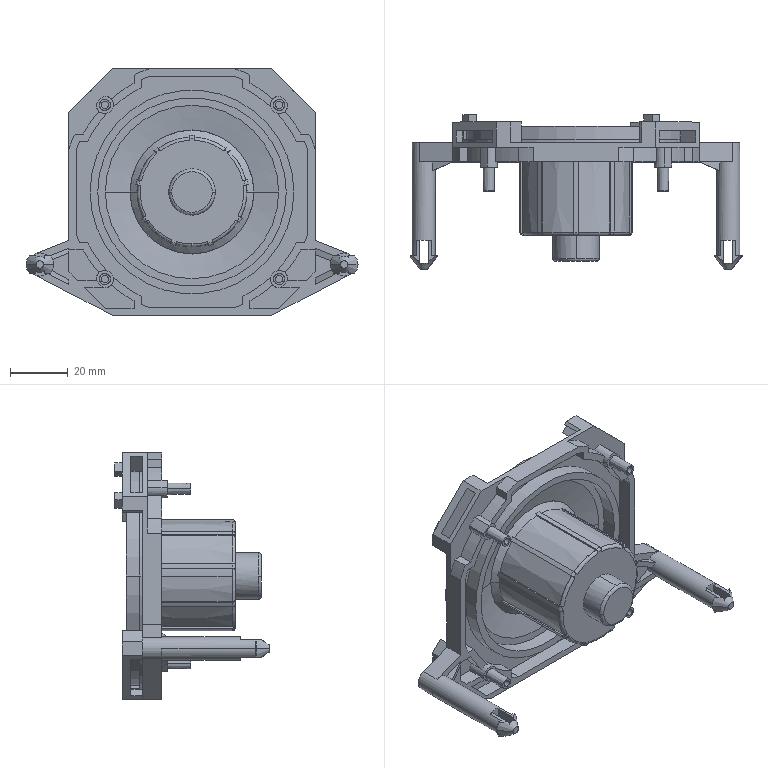Part | STEP file | PINGBITAO_35_15 | 1 solid | 418 faces | box 114.5 x 53.2 x 85 mm | volume 39805 mm3 | plane 212 | cylinder 139 | cone 40 | torus 27 | commonest cylinder face diameters 85 x16 2.5 x12 37.805 x9 39 x9 4.016 x8 8 x8